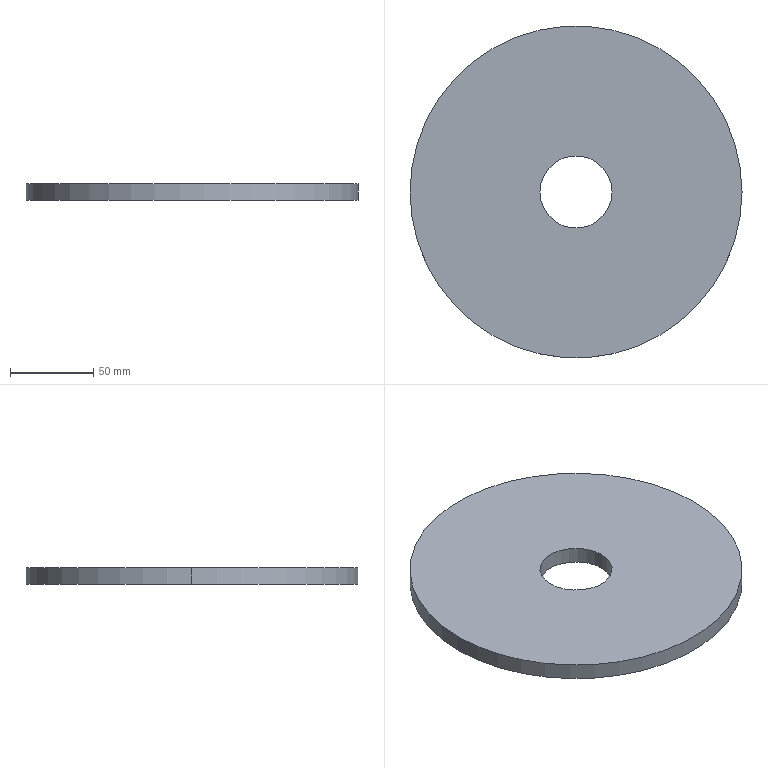Part | SolidWorks | features Extrusion 1 | 1 solid | 6 faces | box 200 x 200 x 10 mm | volume 299298 mm3 | cylinder 4 | plane 2 | commonest cylinder face diameters 43.5 x2 200 x2
STEP:
#1=CARTESIAN_POINT('',(-21.75,0.,10.));
#2=VERTEX_POINT('',#1);
#3=CARTESIAN_POINT('',(21.75,0.,10.));
#4=VERTEX_POINT('',#3);
#5=CARTESIAN_POINT('',(0.,0.,10.));
#6=DIRECTION('',(0.,0.,1.));
#7=DIRECTION('',(1.,0.,0.));
#8=AXIS2_PLACEMENT_3D('',#5,#6,#7);
#9=CIRCLE('',#8,21.75);
#10=EDGE_CURVE('',#2,#4,#9,.T.);
#11=ORIENTED_EDGE('',*,*,#10,.T.);
#12=CARTESIAN_POINT('',(21.75,0.,0.));
#13=VERTEX_POINT('',#12);
#14=CARTESIAN_POINT('',(21.75,0.,10.));
#15=DIRECTION('',(0.,0.,-1.));
#16=VECTOR('',#15,1000.);
#17=LINE('',#14,#16);
#18=EDGE_CURVE('',#4,#13,#17,.T.);
#19=ORIENTED_EDGE('',*,*,#18,.T.);
#20=CARTESIAN_POINT('',(-21.75,0.,0.));
#21=VERTEX_POINT('',#20);
#22=CARTESIAN_POINT('',(0.,0.,0.));
#23=DIRECTION('',(0.,0.,1.));
#24=DIRECTION('',(1.,0.,0.));
#25=AXIS2_PLACEMENT_3D('',#22,#23,#24);
#26=CIRCLE('',#25,21.75);
#27=EDGE_CURVE('',#21,#13,#26,.T.);
#28=ORIENTED_EDGE('',*,*,#27,.F.);
#29=CARTESIAN_POINT('',(-21.75,0.,10.));
#30=DIRECTION('',(0.,0.,-1.));
#31=VECTOR('',#30,1000.);
#32=LINE('',#29,#31);
#33=EDGE_CURVE('',#2,#21,#32,.T.);
#34=ORIENTED_EDGE('',*,*,#33,.F.);
#35=EDGE_LOOP('',(#11,#19,#28,#34));
#36=FACE_OUTER_BOUND('',#35,.T.);
#37=CARTESIAN_POINT('',(0.,0.,10.));
#38=DIRECTION('',(0.,0.,-1.));
#39=DIRECTION('',(-1.,0.,0.));
#40=AXIS2_PLACEMENT_3D('',#37,#38,#39);
#41=CYLINDRICAL_SURFACE('',#40,21.75);
#42=ADVANCED_FACE('',(#36),#41,.F.);
#43=CARTESIAN_POINT('',(100.,0.,10.));
#44=VERTEX_POINT('',#43);
#45=CARTESIAN_POINT('',(-100.,0.,10.));
#46=VERTEX_POINT('',#45);
#47=CARTESIAN_POINT('',(0.,0.,10.));
#48=DIRECTION('',(0.,0.,1.));
#49=DIRECTION('',(1.,0.,0.));
#50=AXIS2_PLACEMENT_3D('',#47,#48,#49);
#51=CIRCLE('',#50,100.);
#52=EDGE_CURVE('',#44,#46,#51,.T.);
#53=ORIENTED_EDGE('',*,*,#52,.F.);
#54=CARTESIAN_POINT('',(100.,0.,0.));
#55=VERTEX_POINT('',#54);
#56=CARTESIAN_POINT('',(100.,0.,10.));
#57=DIRECTION('',(0.,0.,-1.));
#58=VECTOR('',#57,1000.);
#59=LINE('',#56,#58);
#60=EDGE_CURVE('',#44,#55,#59,.T.);
#61=ORIENTED_EDGE('',*,*,#60,.T.);
#62=CARTESIAN_POINT('',(-100.,0.,0.));
#63=VERTEX_POINT('',#62);
#64=CARTESIAN_POINT('',(0.,0.,0.));
#65=DIRECTION('',(0.,0.,1.));
#66=DIRECTION('',(1.,0.,0.));
#67=AXIS2_PLACEMENT_3D('',#64,#65,#66);
#68=CIRCLE('',#67,100.);
#69=EDGE_CURVE('',#55,#63,#68,.T.);
#70=ORIENTED_EDGE('',*,*,#69,.T.);
#71=CARTESIAN_POINT('',(-100.,0.,10.));
#72=DIRECTION('',(0.,0.,-1.));
#73=VECTOR('',#72,1000.);
#74=LINE('',#71,#73);
#75=EDGE_CURVE('',#46,#63,#74,.T.);
#76=ORIENTED_EDGE('',*,*,#75,.F.);
#77=EDGE_LOOP('',(#53,#61,#70,#76));
#78=FACE_OUTER_BOUND('',#77,.T.);
#79=CARTESIAN_POINT('',(0.,0.,10.));
#80=DIRECTION('',(0.,0.,-1.));
#81=DIRECTION('',(-1.,0.,0.));
#82=AXIS2_PLACEMENT_3D('',#79,#80,#81);
#83=CYLINDRICAL_SURFACE('',#82,100.);
#84=ADVANCED_FACE('',(#78),#83,.T.);
#85=CARTESIAN_POINT('',(0.,0.,10.));
#86=DIRECTION('',(0.,0.,1.));
#87=DIRECTION('',(1.,0.,0.));
#88=AXIS2_PLACEMENT_3D('',#85,#86,#87);
#89=CIRCLE('',#88,100.);
#90=EDGE_CURVE('',#46,#44,#89,.T.);
#91=ORIENTED_EDGE('',*,*,#90,.T.);
#92=ORIENTED_EDGE('',*,*,#52,.T.);
#93=EDGE_LOOP('',(#91,#92));
#94=FACE_OUTER_BOUND('',#93,.T.);
#95=ORIENTED_EDGE('',*,*,#10,.F.);
#96=CARTESIAN_POINT('',(0.,0.,10.));
#97=DIRECTION('',(0.,0.,1.));
#98=DIRECTION('',(1.,0.,0.));
#99=AXIS2_PLACEMENT_3D('',#96,#97,#98);
#100=CIRCLE('',#99,21.75);
#101=EDGE_CURVE('',#4,#2,#100,.T.);
#102=ORIENTED_EDGE('',*,*,#101,.F.);
#103=EDGE_LOOP('',(#95,#102));
#104=FACE_BOUND('',#103,.T.);
#105=CARTESIAN_POINT('',(0.,0.,10.));
#106=DIRECTION('',(0.,0.,1.));
#107=DIRECTION('',(1.,0.,0.));
#108=AXIS2_PLACEMENT_3D('',#105,#106,#107);
#109=PLANE('',#108);
#110=ADVANCED_FACE('',(#94,#104),#109,.T.);
#111=CARTESIAN_POINT('',(0.,0.,0.));
#112=DIRECTION('',(0.,0.,1.));
#113=DIRECTION('',(1.,0.,0.));
#114=AXIS2_PLACEMENT_3D('',#111,#112,#113);
#115=CIRCLE('',#114,100.);
#116=EDGE_CURVE('',#63,#55,#115,.T.);
#117=ORIENTED_EDGE('',*,*,#116,.F.);
#118=ORIENTED_EDGE('',*,*,#69,.F.);
#119=EDGE_LOOP('',(#117,#118));
#120=FACE_OUTER_BOUND('',#119,.T.);
#121=ORIENTED_EDGE('',*,*,#27,.T.);
#122=CARTESIAN_POINT('',(0.,0.,0.));
#123=DIRECTION('',(0.,0.,1.));
#124=DIRECTION('',(1.,0.,0.));
#125=AXIS2_PLACEMENT_3D('',#122,#123,#124);
#126=CIRCLE('',#125,21.75);
#127=EDGE_CURVE('',#13,#21,#126,.T.);
#128=ORIENTED_EDGE('',*,*,#127,.T.);
#129=EDGE_LOOP('',(#121,#128));
#130=FACE_BOUND('',#129,.T.);
#131=CARTESIAN_POINT('',(0.,0.,0.));
#132=DIRECTION('',(0.,0.,1.));
#133=DIRECTION('',(1.,0.,0.));
#134=AXIS2_PLACEMENT_3D('',#131,#132,#133);
#135=PLANE('',#134);
#136=ADVANCED_FACE('',(#120,#130),#135,.F.);
#137=ORIENTED_EDGE('',*,*,#60,.F.);
#138=ORIENTED_EDGE('',*,*,#90,.F.);
#139=ORIENTED_EDGE('',*,*,#75,.T.);
#140=ORIENTED_EDGE('',*,*,#116,.T.);
#141=EDGE_LOOP('',(#137,#138,#139,#140));
#142=FACE_OUTER_BOUND('',#141,.T.);
#143=CARTESIAN_POINT('',(0.,0.,10.));
#144=DIRECTION('',(0.,0.,-1.));
#145=DIRECTION('',(-1.,0.,0.));
#146=AXIS2_PLACEMENT_3D('',#143,#144,#145);
#147=CYLINDRICAL_SURFACE('',#146,100.);
#148=ADVANCED_FACE('',(#142),#147,.T.);
#149=ORIENTED_EDGE('',*,*,#18,.F.);
#150=ORIENTED_EDGE('',*,*,#101,.T.);
#151=ORIENTED_EDGE('',*,*,#33,.T.);
#152=ORIENTED_EDGE('',*,*,#127,.F.);
#153=EDGE_LOOP('',(#149,#150,#151,#152));
#154=FACE_OUTER_BOUND('',#153,.T.);
#155=CARTESIAN_POINT('',(0.,0.,10.));
#156=DIRECTION('',(0.,0.,-1.));
#157=DIRECTION('',(-1.,0.,0.));
#158=AXIS2_PLACEMENT_3D('',#155,#156,#157);
#159=CYLINDRICAL_SURFACE('',#158,21.75);
#160=ADVANCED_FACE('',(#154),#159,.F.);
#161=CLOSED_SHELL('',(#42,#84,#110,#136,#148,#160));
#162=MANIFOLD_SOLID_BREP('',#161);
#163=CARTESIAN_POINT('',(0.,0.,0.));
#164=DIRECTION('',(0.,0.,1.));
#165=DIRECTION('',(1.,0.,0.));
#166=AXIS2_PLACEMENT_3D('',#163,#164,#165);
#167=(LENGTH_UNIT()NAMED_UNIT(*)SI_UNIT(.MILLI.,.METRE.));
#168=UNCERTAINTY_MEASURE_WITH_UNIT(LENGTH_MEASURE(0.00001),#167,'','');
#169=(NAMED_UNIT(*)PLANE_ANGLE_UNIT()SI_UNIT($,.RADIAN.));
#170=(NAMED_UNIT(*)SI_UNIT($,.STERADIAN.)SOLID_ANGLE_UNIT());
#171=(GEOMETRIC_REPRESENTATION_CONTEXT(3)GLOBAL_UNCERTAINTY_ASSIGNED_CONTEXT((#168))GLOBAL_UNIT_ASSIGNED_CONTEXT((#167,#169,#170))REPRESENTATION_CONTEXT('',''));
#172=ADVANCED_BREP_SHAPE_REPRESENTATION('',(#162,#166),#171);